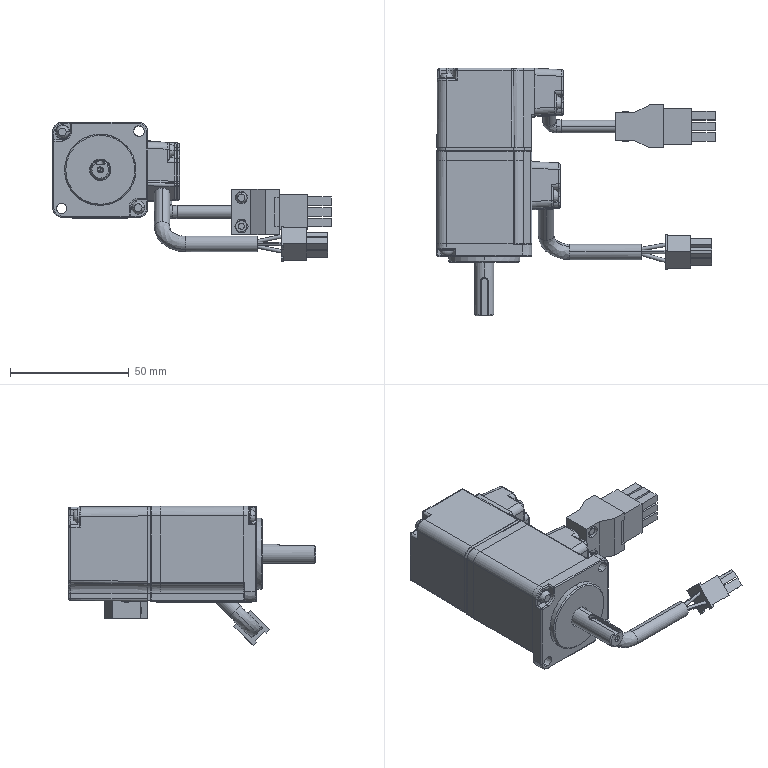Part | SolidWorks | features BaseBody 2 | 2 solids | 689 faces | box 117.111 x 104.2 x 58.651 mm | volume 144018 mm3 | plane 360 | cylinder 186 | spline 73 | cone 42 | torus 28 | commonest cylinder face diameters 2 x67 1 x33 1.5 x11 0.4 x10 3 x9 4 x8